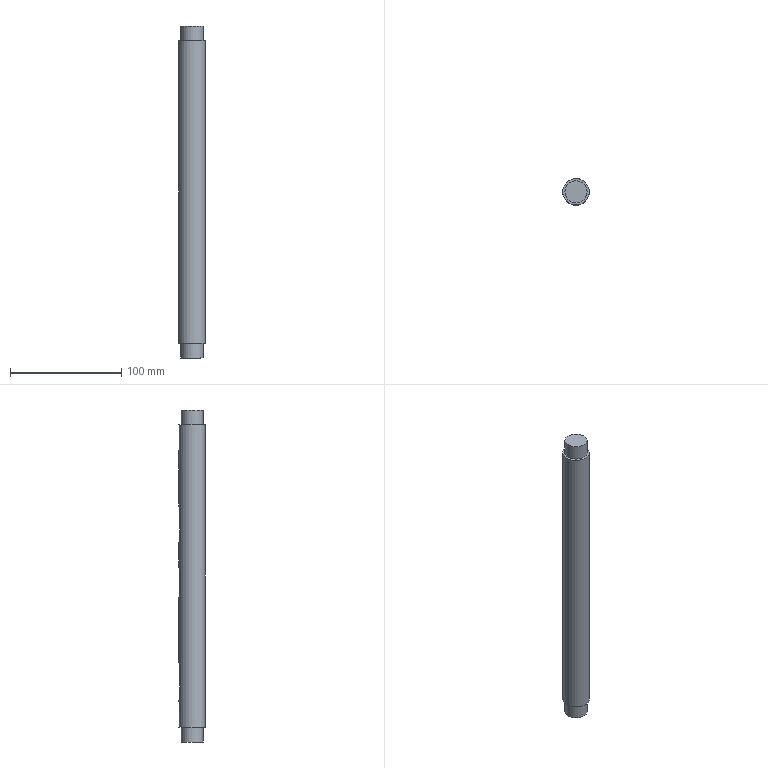Part | NX | features DATUM_CSYS 1, EXTRACT_DATUM_PLANE 1, EXTRUDE 1, SKETCH 1, SWP104 1 | 1 solid | 39 faces | box 23.908 x 23.908 x 299 mm | volume 125501 mm3 | spline 20 | plane 16 | cylinder 3 | commonest cylinder face diameters 19.908 x2 23.908 x1